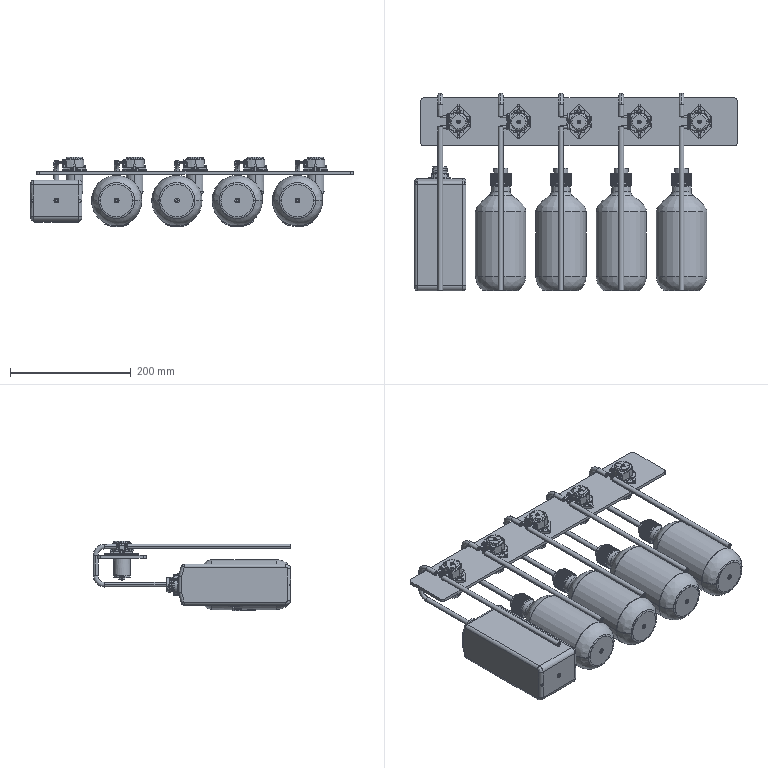Part | SolidWorks | 91 solids | 8483 faces | volume 1784290 mm3 | cylinder 3190 | plane 2410 | spline 1140 | sphere 982 | torus 551 | cone 210 | commonest cylinder face diameters 0.3 x880 0.4 x440 0.2 x140 2 x130 2.515 x130 0.5 x120